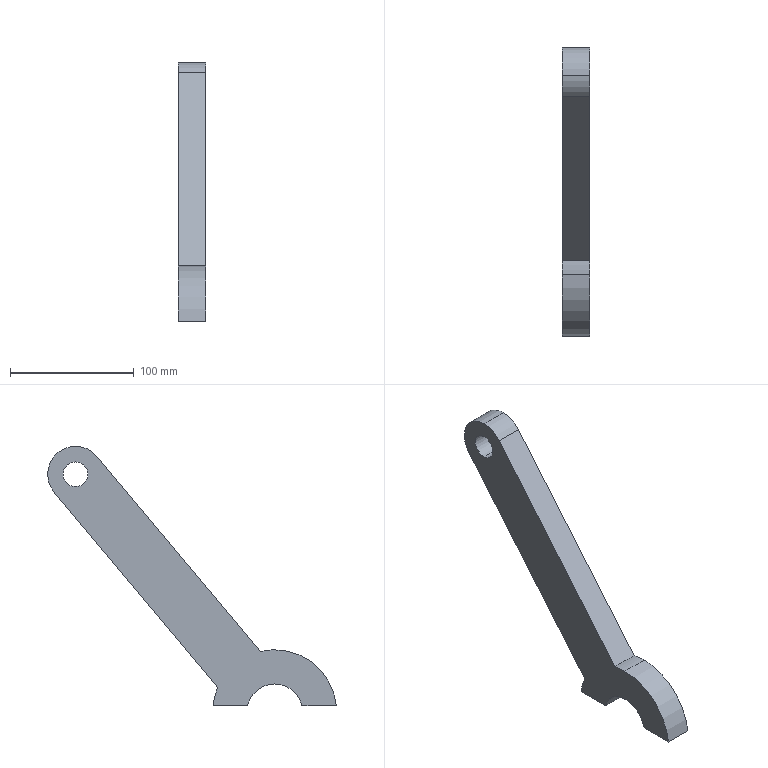Part | SolidWorks | features BaseBody 14, ICE 7, MoveFace 2 | 1 solid | 15 faces | box 22 x 233.027 x 209.178 mm | volume 273312 mm3 | cylinder 9 | plane 6 | commonest cylinder face diameters 45 x4 100 x3 20 x2
STEP:
#1=CARTESIAN_POINT('',(82.124,-77.503,1007.7));
#2=VERTEX_POINT('',#1);
#3=CARTESIAN_POINT('',(82.124,-77.503,1027.7));
#4=VERTEX_POINT('',#3);
#5=CARTESIAN_POINT('',(82.124,-77.503,1017.7));
#6=DIRECTION('',(-1.,0.,0.));
#7=DIRECTION('',(0.,0.,1.));
#8=AXIS2_PLACEMENT_3D('',#5,#6,#7);
#9=CIRCLE('',#8,10.);
#10=EDGE_CURVE('',#2,#4,#9,.T.);
#11=ORIENTED_EDGE('',*,*,#10,.F.);
#12=CARTESIAN_POINT('',(60.124,-77.503,1007.7));
#13=VERTEX_POINT('',#12);
#14=CARTESIAN_POINT('',(82.124,-77.503,1007.7));
#15=DIRECTION('',(-1.,0.,0.));
#16=VECTOR('',#15,1000.);
#17=LINE('',#14,#16);
#18=EDGE_CURVE('',#2,#13,#17,.T.);
#19=ORIENTED_EDGE('',*,*,#18,.T.);
#20=CARTESIAN_POINT('',(60.124,-77.503,1027.7));
#21=VERTEX_POINT('',#20);
#22=CARTESIAN_POINT('',(60.124,-77.503,1017.7));
#23=DIRECTION('',(-1.,0.,0.));
#24=DIRECTION('',(0.,0.,1.));
#25=AXIS2_PLACEMENT_3D('',#22,#23,#24);
#26=CIRCLE('',#25,10.);
#27=EDGE_CURVE('',#13,#21,#26,.T.);
#28=ORIENTED_EDGE('',*,*,#27,.T.);
#29=CARTESIAN_POINT('',(82.124,-77.503,1027.7));
#30=DIRECTION('',(-1.,0.,0.));
#31=VECTOR('',#30,1000.);
#32=LINE('',#29,#31);
#33=EDGE_CURVE('',#4,#21,#32,.T.);
#34=ORIENTED_EDGE('',*,*,#33,.F.);
#35=EDGE_LOOP('',(#11,#19,#28,#34));
#36=FACE_OUTER_BOUND('',#35,.T.);
#37=CARTESIAN_POINT('',(82.124,-77.503,1017.7));
#38=DIRECTION('',(-1.,0.,0.));
#39=DIRECTION('',(0.,0.,1.));
#40=AXIS2_PLACEMENT_3D('',#37,#38,#39);
#41=CYLINDRICAL_SURFACE('',#40,10.);
#42=ADVANCED_FACE('',(#36),#41,.F.);
#43=CARTESIAN_POINT('',(82.124,-216.343,831.023));
#44=VERTEX_POINT('',#43);
#45=CARTESIAN_POINT('',(82.124,-238.28,848.523));
#46=VERTEX_POINT('',#45);
#47=CARTESIAN_POINT('',(82.124,-238.28,826.023));
#48=DIRECTION('',(1.,0.,0.));
#49=DIRECTION('',(0.,0.,-1.));
#50=AXIS2_PLACEMENT_3D('',#47,#48,#49);
#51=CIRCLE('',#50,22.5);
#52=EDGE_CURVE('',#44,#46,#51,.T.);
#53=ORIENTED_EDGE('',*,*,#52,.T.);
#54=CARTESIAN_POINT('',(60.124,-238.28,848.523));
#55=VERTEX_POINT('',#54);
#56=CARTESIAN_POINT('',(191.326,-238.28,848.523));
#57=DIRECTION('',(-1.,0.,0.));
#58=VECTOR('',#57,1000.);
#59=LINE('',#56,#58);
#60=EDGE_CURVE('',#46,#55,#59,.T.);
#61=ORIENTED_EDGE('',*,*,#60,.T.);
#62=CARTESIAN_POINT('',(60.124,-216.343,831.023));
#63=VERTEX_POINT('',#62);
#64=CARTESIAN_POINT('',(60.124,-238.28,826.023));
#65=DIRECTION('',(1.,0.,0.));
#66=DIRECTION('',(0.,0.,1.));
#67=AXIS2_PLACEMENT_3D('',#64,#65,#66);
#68=CIRCLE('',#67,22.5);
#69=EDGE_CURVE('',#63,#55,#68,.T.);
#70=ORIENTED_EDGE('',*,*,#69,.F.);
#71=CARTESIAN_POINT('',(191.326,-216.343,831.023));
#72=DIRECTION('',(-1.,0.,0.));
#73=VECTOR('',#72,1000.);
#74=LINE('',#71,#73);
#75=EDGE_CURVE('',#44,#63,#74,.T.);
#76=ORIENTED_EDGE('',*,*,#75,.F.);
#77=EDGE_LOOP('',(#53,#61,#70,#76));
#78=FACE_OUTER_BOUND('',#77,.T.);
#79=CARTESIAN_POINT('',(191.326,-238.28,826.023));
#80=DIRECTION('',(-1.,0.,0.));
#81=DIRECTION('',(0.,0.,1.));
#82=AXIS2_PLACEMENT_3D('',#79,#80,#81);
#83=CYLINDRICAL_SURFACE('',#82,22.5);
#84=ADVANCED_FACE('',(#78),#83,.F.);
#85=CARTESIAN_POINT('',(82.124,-288.03,831.023));
#86=VERTEX_POINT('',#85);
#87=CARTESIAN_POINT('',(82.124,-238.28,876.023));
#88=VERTEX_POINT('',#87);
#89=CARTESIAN_POINT('',(82.124,-238.28,826.023));
#90=DIRECTION('',(-1.,0.,0.));
#91=DIRECTION('',(0.,0.,-1.));
#92=AXIS2_PLACEMENT_3D('',#89,#90,#91);
#93=CIRCLE('',#92,50.);
#94=EDGE_CURVE('',#86,#88,#93,.T.);
#95=ORIENTED_EDGE('',*,*,#94,.T.);
#96=CARTESIAN_POINT('',(60.124,-238.28,876.023));
#97=VERTEX_POINT('',#96);
#98=CARTESIAN_POINT('',(191.326,-238.28,876.023));
#99=DIRECTION('',(-1.,0.,0.));
#100=VECTOR('',#99,1000.);
#101=LINE('',#98,#100);
#102=EDGE_CURVE('',#88,#97,#101,.T.);
#103=ORIENTED_EDGE('',*,*,#102,.T.);
#104=CARTESIAN_POINT('',(60.124,-288.03,831.023));
#105=VERTEX_POINT('',#104);
#106=CARTESIAN_POINT('',(60.124,-238.28,826.023));
#107=DIRECTION('',(-1.,0.,0.));
#108=DIRECTION('',(0.,0.,1.));
#109=AXIS2_PLACEMENT_3D('',#106,#107,#108);
#110=CIRCLE('',#109,50.);
#111=EDGE_CURVE('',#105,#97,#110,.T.);
#112=ORIENTED_EDGE('',*,*,#111,.F.);
#113=CARTESIAN_POINT('',(191.326,-288.03,831.023));
#114=DIRECTION('',(-1.,0.,0.));
#115=VECTOR('',#114,1000.);
#116=LINE('',#113,#115);
#117=EDGE_CURVE('',#86,#105,#116,.T.);
#118=ORIENTED_EDGE('',*,*,#117,.F.);
#119=EDGE_LOOP('',(#95,#103,#112,#118));
#120=FACE_OUTER_BOUND('',#119,.T.);
#121=CARTESIAN_POINT('',(191.326,-238.28,826.023));
#122=DIRECTION('',(-1.,0.,0.));
#123=DIRECTION('',(0.,0.,1.));
#124=AXIS2_PLACEMENT_3D('',#121,#122,#123);
#125=CYLINDRICAL_SURFACE('',#124,50.);
#126=ADVANCED_FACE('',(#120),#125,.T.);
#127=CARTESIAN_POINT('',(82.124,-94.742,1032.16));
#128=VERTEX_POINT('',#127);
#129=CARTESIAN_POINT('',(82.124,-77.503,1040.2));
#130=VERTEX_POINT('',#129);
#131=CARTESIAN_POINT('',(82.124,-77.503,1017.7));
#132=DIRECTION('',(-1.,0.,0.));
#133=DIRECTION('',(0.,0.,1.));
#134=AXIS2_PLACEMENT_3D('',#131,#132,#133);
#135=CIRCLE('',#134,22.5);
#136=EDGE_CURVE('',#128,#130,#135,.T.);
#137=ORIENTED_EDGE('',*,*,#136,.T.);
#138=CARTESIAN_POINT('',(60.124,-77.503,1040.2));
#139=VERTEX_POINT('',#138);
#140=CARTESIAN_POINT('',(72.124,-77.503,1040.2));
#141=DIRECTION('',(-1.,0.,0.));
#142=VECTOR('',#141,1000.);
#143=LINE('',#140,#142);
#144=EDGE_CURVE('',#130,#139,#143,.T.);
#145=ORIENTED_EDGE('',*,*,#144,.T.);
#146=CARTESIAN_POINT('',(60.124,-94.742,1032.16));
#147=VERTEX_POINT('',#146);
#148=CARTESIAN_POINT('',(60.124,-77.503,1017.7));
#149=DIRECTION('',(1.,0.,0.));
#150=DIRECTION('',(0.,0.,1.));
#151=AXIS2_PLACEMENT_3D('',#148,#149,#150);
#152=CIRCLE('',#151,22.5);
#153=EDGE_CURVE('',#139,#147,#152,.T.);
#154=ORIENTED_EDGE('',*,*,#153,.T.);
#155=CARTESIAN_POINT('',(72.124,-94.742,1032.16));
#156=DIRECTION('',(1.,0.,0.));
#157=VECTOR('',#156,1000.);
#158=LINE('',#155,#157);
#159=EDGE_CURVE('',#147,#128,#158,.T.);
#160=ORIENTED_EDGE('',*,*,#159,.T.);
#161=EDGE_LOOP('',(#137,#145,#154,#160));
#162=FACE_OUTER_BOUND('',#161,.T.);
#163=CARTESIAN_POINT('',(72.124,-77.503,1017.7));
#164=DIRECTION('',(-1.,0.,0.));
#165=DIRECTION('',(0.,0.,1.));
#166=AXIS2_PLACEMENT_3D('',#163,#164,#165);
#167=CYLINDRICAL_SURFACE('',#166,22.5);
#168=ADVANCED_FACE('',(#162),#167,.T.);
#169=ORIENTED_EDGE('',*,*,#144,.F.);
#170=CARTESIAN_POINT('',(82.124,-60.265,1003.241));
#171=VERTEX_POINT('',#170);
#172=CARTESIAN_POINT('',(82.124,-77.503,1017.7));
#173=DIRECTION('',(-1.,0.,0.));
#174=DIRECTION('',(0.,0.,1.));
#175=AXIS2_PLACEMENT_3D('',#172,#173,#174);
#176=CIRCLE('',#175,22.5);
#177=EDGE_CURVE('',#130,#171,#176,.T.);
#178=ORIENTED_EDGE('',*,*,#177,.T.);
#179=CARTESIAN_POINT('',(60.124,-60.265,1003.241));
#180=VERTEX_POINT('',#179);
#181=CARTESIAN_POINT('',(72.124,-60.265,1003.241));
#182=DIRECTION('',(-1.,0.,0.));
#183=VECTOR('',#182,1000.);
#184=LINE('',#181,#183);
#185=EDGE_CURVE('',#171,#180,#184,.T.);
#186=ORIENTED_EDGE('',*,*,#185,.T.);
#187=CARTESIAN_POINT('',(60.124,-77.503,1017.7));
#188=DIRECTION('',(1.,0.,0.));
#189=DIRECTION('',(0.,0.,1.));
#190=AXIS2_PLACEMENT_3D('',#187,#188,#189);
#191=CIRCLE('',#190,22.5);
#192=EDGE_CURVE('',#180,#139,#191,.T.);
#193=ORIENTED_EDGE('',*,*,#192,.T.);
#194=EDGE_LOOP('',(#169,#178,#186,#193));
#195=FACE_OUTER_BOUND('',#194,.T.);
#196=CARTESIAN_POINT('',(72.124,-77.503,1017.7));
#197=DIRECTION('',(-1.,0.,0.));
#198=DIRECTION('',(0.,0.,1.));
#199=AXIS2_PLACEMENT_3D('',#196,#197,#198);
#200=CYLINDRICAL_SURFACE('',#199,22.5);
#201=ADVANCED_FACE('',(#195),#200,.T.);
#202=CARTESIAN_POINT('',(60.124,-77.503,1017.7));
#203=DIRECTION('',(-1.,0.,0.));
#204=DIRECTION('',(0.,0.,1.));
#205=AXIS2_PLACEMENT_3D('',#202,#203,#204);
#206=CIRCLE('',#205,10.);
#207=EDGE_CURVE('',#21,#13,#206,.T.);
#208=ORIENTED_EDGE('',*,*,#207,.F.);
#209=ORIENTED_EDGE('',*,*,#27,.F.);
#210=EDGE_LOOP('',(#208,#209));
#211=FACE_BOUND('',#210,.T.);
#212=CARTESIAN_POINT('',(60.124,-192.347,845.773));
#213=VERTEX_POINT('',#212);
#214=CARTESIAN_POINT('',(60.124,-188.531,831.023));
#215=VERTEX_POINT('',#214);
#216=CARTESIAN_POINT('',(60.124,-238.28,826.023));
#217=DIRECTION('',(-1.,0.,0.));
#218=DIRECTION('',(0.,0.,1.));
#219=AXIS2_PLACEMENT_3D('',#216,#217,#218);
#220=CIRCLE('',#219,50.);
#221=EDGE_CURVE('',#213,#215,#220,.T.);
#222=ORIENTED_EDGE('',*,*,#221,.T.);
#223=CARTESIAN_POINT('',(60.124,-216.343,831.023));
#224=DIRECTION('',(0.,-1.,0.));
#225=VECTOR('',#224,1000.);
#226=LINE('',#223,#225);
#227=EDGE_CURVE('',#215,#63,#226,.T.);
#228=ORIENTED_EDGE('',*,*,#227,.T.);
#229=ORIENTED_EDGE('',*,*,#69,.T.);
#230=CARTESIAN_POINT('',(60.124,-260.218,831.023));
#231=VERTEX_POINT('',#230);
#232=CARTESIAN_POINT('',(60.124,-238.28,826.023));
#233=DIRECTION('',(1.,0.,0.));
#234=DIRECTION('',(0.,0.,1.));
#235=AXIS2_PLACEMENT_3D('',#232,#233,#234);
#236=CIRCLE('',#235,22.5);
#237=EDGE_CURVE('',#55,#231,#236,.T.);
#238=ORIENTED_EDGE('',*,*,#237,.T.);
#239=CARTESIAN_POINT('',(60.124,-288.03,831.023));
#240=DIRECTION('',(0.,-1.,0.));
#241=VECTOR('',#240,1000.);
#242=LINE('',#239,#241);
#243=EDGE_CURVE('',#231,#105,#242,.T.);
#244=ORIENTED_EDGE('',*,*,#243,.T.);
#245=ORIENTED_EDGE('',*,*,#111,.T.);
#246=CARTESIAN_POINT('',(60.124,-226.824,874.692));
#247=VERTEX_POINT('',#246);
#248=CARTESIAN_POINT('',(60.124,-238.28,826.023));
#249=DIRECTION('',(-1.,0.,0.));
#250=DIRECTION('',(0.,0.,1.));
#251=AXIS2_PLACEMENT_3D('',#248,#249,#250);
#252=CIRCLE('',#251,50.);
#253=EDGE_CURVE('',#97,#247,#252,.T.);
#254=ORIENTED_EDGE('',*,*,#253,.T.);
#255=CARTESIAN_POINT('',(60.124,-94.742,1032.16));
#256=DIRECTION('',(0.,-0.6426,-0.7662));
#257=VECTOR('',#256,1000.);
#258=LINE('',#255,#257);
#259=EDGE_CURVE('',#147,#247,#258,.T.);
#260=ORIENTED_EDGE('',*,*,#259,.F.);
#261=ORIENTED_EDGE('',*,*,#153,.F.);
#262=ORIENTED_EDGE('',*,*,#192,.F.);
#263=CARTESIAN_POINT('',(60.124,-208.913,826.023));
#264=DIRECTION('',(0.,0.6426,0.7662));
#265=VECTOR('',#264,1000.);
#266=LINE('',#263,#265);
#267=EDGE_CURVE('',#213,#180,#266,.T.);
#268=ORIENTED_EDGE('',*,*,#267,.F.);
#269=EDGE_LOOP('',(#222,#228,#229,#238,#244,#245,#254,#260,#261,#262,#268));
#270=FACE_OUTER_BOUND('',#269,.T.);
#271=CARTESIAN_POINT('',(60.124,-77.503,1017.7));
#272=DIRECTION('',(1.,0.,0.));
#273=DIRECTION('',(0.,0.,-1.));
#274=AXIS2_PLACEMENT_3D('',#271,#272,#273);
#275=PLANE('',#274);
#276=ADVANCED_FACE('',(#211,#270),#275,.F.);
#277=CARTESIAN_POINT('',(82.124,-192.347,845.773));
#278=VERTEX_POINT('',#277);
#279=CARTESIAN_POINT('',(82.124,-60.265,1003.241));
#280=DIRECTION('',(0.,0.6426,0.7662));
#281=VECTOR('',#280,1000.);
#282=LINE('',#279,#281);
#283=EDGE_CURVE('',#278,#171,#282,.T.);
#284=ORIENTED_EDGE('',*,*,#283,.F.);
#285=CARTESIAN_POINT('',(590.124,-192.347,845.773));
#286=DIRECTION('',(-1.,0.,0.));
#287=VECTOR('',#286,1000.);
#288=LINE('',#285,#287);
#289=EDGE_CURVE('',#278,#213,#288,.T.);
#290=ORIENTED_EDGE('',*,*,#289,.T.);
#291=ORIENTED_EDGE('',*,*,#267,.T.);
#292=ORIENTED_EDGE('',*,*,#185,.F.);
#293=EDGE_LOOP('',(#284,#290,#291,#292));
#294=FACE_OUTER_BOUND('',#293,.T.);
#295=CARTESIAN_POINT('',(72.124,-60.265,1003.241));
#296=DIRECTION('',(0.,-0.7662,0.6426));
#297=DIRECTION('',(0.,-0.6426,-0.7662));
#298=AXIS2_PLACEMENT_3D('',#295,#296,#297);
#299=PLANE('',#298);
#300=ADVANCED_FACE('',(#294),#299,.F.);
#301=ORIENTED_EDGE('',*,*,#259,.T.);
#302=CARTESIAN_POINT('',(82.124,-226.824,874.692));
#303=VERTEX_POINT('',#302);
#304=CARTESIAN_POINT('',(590.124,-226.824,874.692));
#305=DIRECTION('',(1.,0.,0.));
#306=VECTOR('',#305,1000.);
#307=LINE('',#304,#306);
#308=EDGE_CURVE('',#247,#303,#307,.T.);
#309=ORIENTED_EDGE('',*,*,#308,.T.);
#310=CARTESIAN_POINT('',(82.124,-94.742,1032.16));
#311=DIRECTION('',(0.,-0.6426,-0.7662));
#312=VECTOR('',#311,1000.);
#313=LINE('',#310,#312);
#314=EDGE_CURVE('',#128,#303,#313,.T.);
#315=ORIENTED_EDGE('',*,*,#314,.F.);
#316=ORIENTED_EDGE('',*,*,#159,.F.);
#317=EDGE_LOOP('',(#301,#309,#315,#316));
#318=FACE_OUTER_BOUND('',#317,.T.);
#319=CARTESIAN_POINT('',(72.124,-94.742,1032.16));
#320=DIRECTION('',(0.,0.7662,-0.6426));
#321=DIRECTION('',(0.,0.6426,0.7662));
#322=AXIS2_PLACEMENT_3D('',#319,#320,#321);
#323=PLANE('',#322);
#324=ADVANCED_FACE('',(#318),#323,.F.);
#325=CARTESIAN_POINT('',(82.124,-77.503,1017.7));
#326=DIRECTION('',(-1.,0.,0.));
#327=DIRECTION('',(0.,0.,1.));
#328=AXIS2_PLACEMENT_3D('',#325,#326,#327);
#329=CIRCLE('',#328,10.);
#330=EDGE_CURVE('',#4,#2,#329,.T.);
#331=ORIENTED_EDGE('',*,*,#330,.T.);
#332=ORIENTED_EDGE('',*,*,#10,.T.);
#333=EDGE_LOOP('',(#331,#332));
#334=FACE_BOUND('',#333,.T.);
#335=ORIENTED_EDGE('',*,*,#314,.T.);
#336=CARTESIAN_POINT('',(82.124,-238.28,826.023));
#337=DIRECTION('',(-1.,0.,0.));
#338=DIRECTION('',(0.,0.,-1.));
#339=AXIS2_PLACEMENT_3D('',#336,#337,#338);
#340=CIRCLE('',#339,50.);
#341=EDGE_CURVE('',#88,#303,#340,.T.);
#342=ORIENTED_EDGE('',*,*,#341,.F.);
#343=ORIENTED_EDGE('',*,*,#94,.F.);
#344=CARTESIAN_POINT('',(82.124,-260.218,831.023));
#345=VERTEX_POINT('',#344);
#346=CARTESIAN_POINT('',(82.124,-288.03,831.023));
#347=DIRECTION('',(0.,-1.,0.));
#348=VECTOR('',#347,1000.);
#349=LINE('',#346,#348);
#350=EDGE_CURVE('',#345,#86,#349,.T.);
#351=ORIENTED_EDGE('',*,*,#350,.F.);
#352=CARTESIAN_POINT('',(82.124,-238.28,826.023));
#353=DIRECTION('',(1.,0.,0.));
#354=DIRECTION('',(0.,0.,-1.));
#355=AXIS2_PLACEMENT_3D('',#352,#353,#354);
#356=CIRCLE('',#355,22.5);
#357=EDGE_CURVE('',#46,#345,#356,.T.);
#358=ORIENTED_EDGE('',*,*,#357,.F.);
#359=ORIENTED_EDGE('',*,*,#52,.F.);
#360=CARTESIAN_POINT('',(82.124,-188.531,831.023));
#361=VERTEX_POINT('',#360);
#362=CARTESIAN_POINT('',(82.124,-216.343,831.023));
#363=DIRECTION('',(0.,-1.,0.));
#364=VECTOR('',#363,1000.);
#365=LINE('',#362,#364);
#366=EDGE_CURVE('',#361,#44,#365,.T.);
#367=ORIENTED_EDGE('',*,*,#366,.F.);
#368=CARTESIAN_POINT('',(82.124,-238.28,826.023));
#369=DIRECTION('',(-1.,0.,0.));
#370=DIRECTION('',(0.,0.,-1.));
#371=AXIS2_PLACEMENT_3D('',#368,#369,#370);
#372=CIRCLE('',#371,50.);
#373=EDGE_CURVE('',#278,#361,#372,.T.);
#374=ORIENTED_EDGE('',*,*,#373,.F.);
#375=ORIENTED_EDGE('',*,*,#283,.T.);
#376=ORIENTED_EDGE('',*,*,#177,.F.);
#377=ORIENTED_EDGE('',*,*,#136,.F.);
#378=EDGE_LOOP('',(#335,#342,#343,#351,#358,#359,#367,#374,#375,#376,#377));
#379=FACE_OUTER_BOUND('',#378,.T.);
#380=CARTESIAN_POINT('',(82.124,-77.503,1017.7));
#381=DIRECTION('',(1.,0.,0.));
#382=DIRECTION('',(0.,0.,-1.));
#383=AXIS2_PLACEMENT_3D('',#380,#381,#382);
#384=PLANE('',#383);
#385=ADVANCED_FACE('',(#334,#379),#384,.T.);
#386=ORIENTED_EDGE('',*,*,#289,.F.);
#387=ORIENTED_EDGE('',*,*,#373,.T.);
#388=CARTESIAN_POINT('',(191.326,-188.531,831.023));
#389=DIRECTION('',(-1.,0.,0.));
#390=VECTOR('',#389,1000.);
#391=LINE('',#388,#390);
#392=EDGE_CURVE('',#361,#215,#391,.T.);
#393=ORIENTED_EDGE('',*,*,#392,.T.);
#394=ORIENTED_EDGE('',*,*,#221,.F.);
#395=EDGE_LOOP('',(#386,#387,#393,#394));
#396=FACE_OUTER_BOUND('',#395,.T.);
#397=CARTESIAN_POINT('',(191.326,-238.28,826.023));
#398=DIRECTION('',(-1.,0.,0.));
#399=DIRECTION('',(0.,0.,1.));
#400=AXIS2_PLACEMENT_3D('',#397,#398,#399);
#401=CYLINDRICAL_SURFACE('',#400,50.);
#402=ADVANCED_FACE('',(#396),#401,.T.);
#403=ORIENTED_EDGE('',*,*,#102,.F.);
#404=ORIENTED_EDGE('',*,*,#341,.T.);
#405=ORIENTED_EDGE('',*,*,#308,.F.);
#406=ORIENTED_EDGE('',*,*,#253,.F.);
#407=EDGE_LOOP('',(#403,#404,#405,#406));
#408=FACE_OUTER_BOUND('',#407,.T.);
#409=CARTESIAN_POINT('',(191.326,-238.28,826.023));
#410=DIRECTION('',(-1.,0.,0.));
#411=DIRECTION('',(0.,0.,1.));
#412=AXIS2_PLACEMENT_3D('',#409,#410,#411);
#413=CYLINDRICAL_SURFACE('',#412,50.);
#414=ADVANCED_FACE('',(#408),#413,.T.);
#415=CARTESIAN_POINT('',(191.326,-260.218,831.023));
#416=DIRECTION('',(-1.,0.,0.));
#417=VECTOR('',#416,1000.);
#418=LINE('',#415,#417);
#419=EDGE_CURVE('',#345,#231,#418,.T.);
#420=ORIENTED_EDGE('',*,*,#419,.F.);
#421=ORIENTED_EDGE('',*,*,#350,.T.);
#422=ORIENTED_EDGE('',*,*,#117,.T.);
#423=ORIENTED_EDGE('',*,*,#243,.F.);
#424=EDGE_LOOP('',(#420,#421,#422,#423));
#425=FACE_OUTER_BOUND('',#424,.T.);
#426=CARTESIAN_POINT('',(191.326,-288.03,831.023));
#427=DIRECTION('',(0.,0.,-1.));
#428=DIRECTION('',(-1.,0.,0.));
#429=AXIS2_PLACEMENT_3D('',#426,#427,#428);
#430=PLANE('',#429);
#431=ADVANCED_FACE('',(#425),#430,.T.);
#432=ORIENTED_EDGE('',*,*,#392,.F.);
#433=ORIENTED_EDGE('',*,*,#366,.T.);
#434=ORIENTED_EDGE('',*,*,#75,.T.);
#435=ORIENTED_EDGE('',*,*,#227,.F.);
#436=EDGE_LOOP('',(#432,#433,#434,#435));
#437=FACE_OUTER_BOUND('',#436,.T.);
#438=CARTESIAN_POINT('',(191.326,-216.343,831.023));
#439=DIRECTION('',(0.,0.,-1.));
#440=DIRECTION('',(-1.,0.,0.));
#441=AXIS2_PLACEMENT_3D('',#438,#439,#440);
#442=PLANE('',#441);
#443=ADVANCED_FACE('',(#437),#442,.T.);
#444=ORIENTED_EDGE('',*,*,#60,.F.);
#445=ORIENTED_EDGE('',*,*,#357,.T.);
#446=ORIENTED_EDGE('',*,*,#419,.T.);
#447=ORIENTED_EDGE('',*,*,#237,.F.);
#448=EDGE_LOOP('',(#444,#445,#446,#447));
#449=FACE_OUTER_BOUND('',#448,.T.);
#450=CARTESIAN_POINT('',(191.326,-238.28,826.023));
#451=DIRECTION('',(-1.,0.,0.));
#452=DIRECTION('',(0.,0.,1.));
#453=AXIS2_PLACEMENT_3D('',#450,#451,#452);
#454=CYLINDRICAL_SURFACE('',#453,22.5);
#455=ADVANCED_FACE('',(#449),#454,.F.);
#456=ORIENTED_EDGE('',*,*,#18,.F.);
#457=ORIENTED_EDGE('',*,*,#330,.F.);
#458=ORIENTED_EDGE('',*,*,#33,.T.);
#459=ORIENTED_EDGE('',*,*,#207,.T.);
#460=EDGE_LOOP('',(#456,#457,#458,#459));
#461=FACE_OUTER_BOUND('',#460,.T.);
#462=CARTESIAN_POINT('',(82.124,-77.503,1017.7));
#463=DIRECTION('',(-1.,0.,0.));
#464=DIRECTION('',(0.,0.,1.));
#465=AXIS2_PLACEMENT_3D('',#462,#463,#464);
#466=CYLINDRICAL_SURFACE('',#465,10.);
#467=ADVANCED_FACE('',(#461),#466,.F.);
#468=CLOSED_SHELL('',(#42,#84,#126,#168,#201,#276,#300,#324,#385,#402,#414,#431,#443,#455,#467));
#469=MANIFOLD_SOLID_BREP('',#468);
#470=CARTESIAN_POINT('',(0.,0.,0.));
#471=DIRECTION('',(0.,0.,1.));
#472=DIRECTION('',(1.,0.,0.));
#473=AXIS2_PLACEMENT_3D('',#470,#471,#472);
#474=(LENGTH_UNIT()NAMED_UNIT(*)SI_UNIT(.MILLI.,.METRE.));
#475=UNCERTAINTY_MEASURE_WITH_UNIT(LENGTH_MEASURE(0.00001),#474,'','');
#476=(NAMED_UNIT(*)PLANE_ANGLE_UNIT()SI_UNIT($,.RADIAN.));
#477=(NAMED_UNIT(*)SI_UNIT($,.STERADIAN.)SOLID_ANGLE_UNIT());
#478=(GEOMETRIC_REPRESENTATION_CONTEXT(3)GLOBAL_UNCERTAINTY_ASSIGNED_CONTEXT((#475))GLOBAL_UNIT_ASSIGNED_CONTEXT((#474,#476,#477))REPRESENTATION_CONTEXT('',''));
#479=ADVANCED_BREP_SHAPE_REPRESENTATION('',(#469,#473),#478);